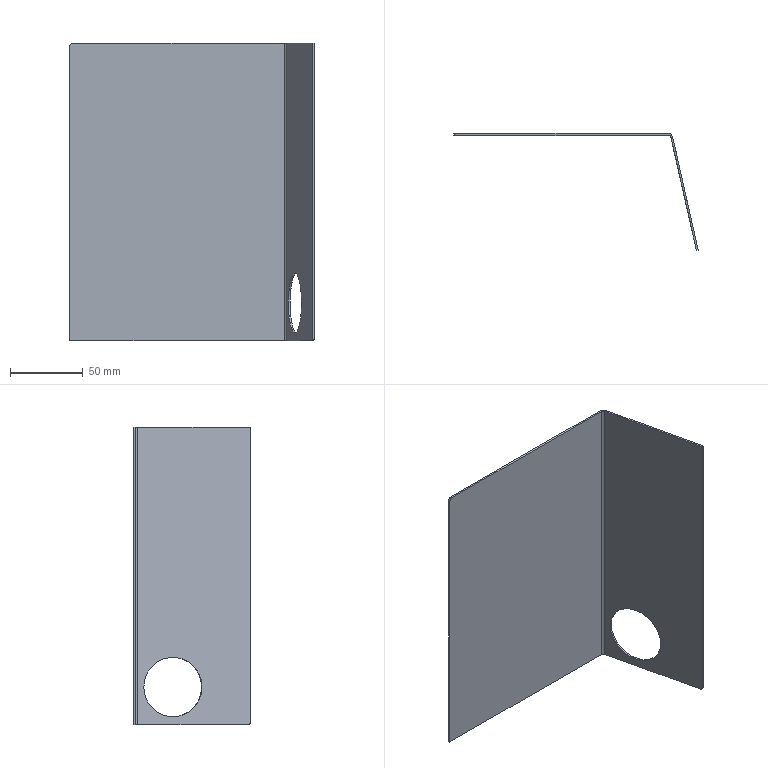Part | SolidWorks | features Fillet 1, FlatPattern 1, ICE 1, SMBaseFlange 1, SheetMetal 1 | 1 solid | 18 faces | box 168 x 80.263 x 204.8 mm | volume 55034 mm3 | plane 12 | cylinder 6 | commonest cylinder face diameters 4 x3 41 x2 6.4 x1
STEP:
#1=CARTESIAN_POINT('',(150.344,-6.995,26.));
#2=VERTEX_POINT('',#1);
#3=CARTESIAN_POINT('',(159.344,-46.995,26.));
#4=VERTEX_POINT('',#3);
#5=CARTESIAN_POINT('',(154.844,-26.995,26.));
#6=DIRECTION('',(-0.9756,-0.2195,0.));
#7=DIRECTION('',(-0.2195,0.9756,0.));
#8=AXIS2_PLACEMENT_3D('',#5,#6,#7);
#9=CIRCLE('',#8,20.5);
#10=EDGE_CURVE('',#2,#4,#9,.T.);
#11=ORIENTED_EDGE('',*,*,#10,.T.);
#12=CARTESIAN_POINT('',(160.515,-46.732,26.));
#13=VERTEX_POINT('',#12);
#14=CARTESIAN_POINT('',(0.5522,-82.723,26.));
#15=DIRECTION('',(0.9756,0.2195,0.));
#16=VECTOR('',#15,1000.);
#17=LINE('',#14,#16);
#18=EDGE_CURVE('',#4,#13,#17,.T.);
#19=ORIENTED_EDGE('',*,*,#18,.T.);
#20=CARTESIAN_POINT('',(151.515,-6.732,26.));
#21=VERTEX_POINT('',#20);
#22=CARTESIAN_POINT('',(156.015,-26.732,26.));
#23=DIRECTION('',(0.9756,0.2195,0.));
#24=DIRECTION('',(-0.2195,0.9756,0.));
#25=AXIS2_PLACEMENT_3D('',#22,#23,#24);
#26=CIRCLE('',#25,20.5);
#27=EDGE_CURVE('',#13,#21,#26,.T.);
#28=ORIENTED_EDGE('',*,*,#27,.T.);
#29=CARTESIAN_POINT('',(-8.448,-42.723,26.));
#30=DIRECTION('',(0.9756,0.2195,0.));
#31=VECTOR('',#30,1000.);
#32=LINE('',#29,#31);
#33=EDGE_CURVE('',#2,#21,#32,.T.);
#34=ORIENTED_EDGE('',*,*,#33,.F.);
#35=EDGE_LOOP('',(#11,#19,#28,#34));
#36=FACE_OUTER_BOUND('',#35,.T.);
#37=CARTESIAN_POINT('',(-3.948,-62.723,26.));
#38=DIRECTION('',(0.9756,0.2195,0.));
#39=DIRECTION('',(-0.2195,0.9756,0.));
#40=AXIS2_PLACEMENT_3D('',#37,#38,#39);
#41=CYLINDRICAL_SURFACE('',#40,20.5);
#42=ADVANCED_FACE('',(#36),#41,.F.);
#43=CARTESIAN_POINT('',(150.562,-2.498,204.8));
#44=VERTEX_POINT('',#43);
#45=CARTESIAN_POINT('',(149.391,-2.761,204.8));
#46=VERTEX_POINT('',#45);
#47=CARTESIAN_POINT('',(150.562,-2.498,204.8));
#48=DIRECTION('',(-0.9756,-0.2195,0.));
#49=VECTOR('',#48,1000.);
#50=LINE('',#47,#49);
#51=EDGE_CURVE('',#44,#46,#50,.T.);
#52=ORIENTED_EDGE('',*,*,#51,.F.);
#53=CARTESIAN_POINT('',(147.44,0.,204.8));
#54=VERTEX_POINT('',#53);
#55=CARTESIAN_POINT('',(147.44,-3.2,204.8));
#56=DIRECTION('',(0.,0.,-1.));
#57=DIRECTION('',(1.,0.,0.));
#58=AXIS2_PLACEMENT_3D('',#55,#56,#57);
#59=CIRCLE('',#58,3.2);
#60=EDGE_CURVE('',#54,#44,#59,.T.);
#61=ORIENTED_EDGE('',*,*,#60,.F.);
#62=CARTESIAN_POINT('',(147.44,-1.2,204.8));
#63=VERTEX_POINT('',#62);
#64=CARTESIAN_POINT('',(147.44,-1.2,204.8));
#65=DIRECTION('',(0.,1.,0.));
#66=VECTOR('',#65,1000.);
#67=LINE('',#64,#66);
#68=EDGE_CURVE('',#63,#54,#67,.T.);
#69=ORIENTED_EDGE('',*,*,#68,.F.);
#70=CARTESIAN_POINT('',(147.44,-3.2,204.8));
#71=DIRECTION('',(0.,0.,-1.));
#72=DIRECTION('',(1.,0.,0.));
#73=AXIS2_PLACEMENT_3D('',#70,#71,#72);
#74=CIRCLE('',#73,2.);
#75=EDGE_CURVE('',#63,#46,#74,.T.);
#76=ORIENTED_EDGE('',*,*,#75,.T.);
#77=EDGE_LOOP('',(#52,#61,#69,#76));
#78=FACE_OUTER_BOUND('',#77,.T.);
#79=CARTESIAN_POINT('',(150.562,-2.498,204.8));
#80=DIRECTION('',(0.,0.,1.));
#81=DIRECTION('',(1.,0.,0.));
#82=AXIS2_PLACEMENT_3D('',#79,#80,#81);
#83=PLANE('',#82);
#84=ADVANCED_FACE('',(#78),#83,.T.);
#85=CARTESIAN_POINT('',(168.,-80.,204.8));
#86=VERTEX_POINT('',#85);
#87=CARTESIAN_POINT('',(150.,0.,204.8));
#88=DIRECTION('',(0.2195,-0.9756,0.));
#89=VECTOR('',#88,1000.);
#90=LINE('',#87,#89);
#91=EDGE_CURVE('',#44,#86,#90,.T.);
#92=ORIENTED_EDGE('',*,*,#91,.F.);
#93=ORIENTED_EDGE('',*,*,#51,.T.);
#94=CARTESIAN_POINT('',(166.829,-80.263,204.8));
#95=VERTEX_POINT('',#94);
#96=CARTESIAN_POINT('',(148.829,-0.2634,204.8));
#97=DIRECTION('',(0.2195,-0.9756,0.));
#98=VECTOR('',#97,1000.);
#99=LINE('',#96,#98);
#100=EDGE_CURVE('',#46,#95,#99,.T.);
#101=ORIENTED_EDGE('',*,*,#100,.T.);
#102=CARTESIAN_POINT('',(168.,-80.,204.8));
#103=DIRECTION('',(-0.9756,-0.2195,0.));
#104=VECTOR('',#103,1000.);
#105=LINE('',#102,#104);
#106=EDGE_CURVE('',#86,#95,#105,.T.);
#107=ORIENTED_EDGE('',*,*,#106,.F.);
#108=EDGE_LOOP('',(#92,#93,#101,#107));
#109=FACE_OUTER_BOUND('',#108,.T.);
#110=CARTESIAN_POINT('',(147.44,-1.2,204.8));
#111=DIRECTION('',(0.,0.,1.));
#112=DIRECTION('',(1.,0.,0.));
#113=AXIS2_PLACEMENT_3D('',#110,#111,#112);
#114=PLANE('',#113);
#115=ADVANCED_FACE('',(#109),#114,.T.);
#116=CARTESIAN_POINT('',(147.44,0.,0.));
#117=VERTEX_POINT('',#116);
#118=CARTESIAN_POINT('',(147.44,-1.2,0.));
#119=VERTEX_POINT('',#118);
#120=CARTESIAN_POINT('',(147.44,0.,0.));
#121=DIRECTION('',(0.,-1.,0.));
#122=VECTOR('',#121,1000.);
#123=LINE('',#120,#122);
#124=EDGE_CURVE('',#117,#119,#123,.T.);
#125=ORIENTED_EDGE('',*,*,#124,.F.);
#126=CARTESIAN_POINT('',(150.562,-2.498,0.));
#127=VERTEX_POINT('',#126);
#128=CARTESIAN_POINT('',(147.44,-3.2,0.));
#129=DIRECTION('',(0.,0.,-1.));
#130=DIRECTION('',(1.,0.,0.));
#131=AXIS2_PLACEMENT_3D('',#128,#129,#130);
#132=CIRCLE('',#131,3.2);
#133=EDGE_CURVE('',#117,#127,#132,.T.);
#134=ORIENTED_EDGE('',*,*,#133,.T.);
#135=CARTESIAN_POINT('',(149.391,-2.761,0.));
#136=VERTEX_POINT('',#135);
#137=CARTESIAN_POINT('',(149.391,-2.761,0.));
#138=DIRECTION('',(0.9756,0.2195,0.));
#139=VECTOR('',#138,1000.);
#140=LINE('',#137,#139);
#141=EDGE_CURVE('',#136,#127,#140,.T.);
#142=ORIENTED_EDGE('',*,*,#141,.F.);
#143=CARTESIAN_POINT('',(147.44,-3.2,0.));
#144=DIRECTION('',(0.,0.,-1.));
#145=DIRECTION('',(1.,0.,0.));
#146=AXIS2_PLACEMENT_3D('',#143,#144,#145);
#147=CIRCLE('',#146,2.);
#148=EDGE_CURVE('',#119,#136,#147,.T.);
#149=ORIENTED_EDGE('',*,*,#148,.F.);
#150=EDGE_LOOP('',(#125,#134,#142,#149));
#151=FACE_OUTER_BOUND('',#150,.T.);
#152=CARTESIAN_POINT('',(147.44,0.,0.));
#153=DIRECTION('',(0.,0.,-1.));
#154=DIRECTION('',(-1.,0.,0.));
#155=AXIS2_PLACEMENT_3D('',#152,#153,#154);
#156=PLANE('',#155);
#157=ADVANCED_FACE('',(#151),#156,.T.);
#158=CARTESIAN_POINT('',(0.,0.,0.));
#159=VERTEX_POINT('',#158);
#160=CARTESIAN_POINT('',(0.,0.,0.));
#161=DIRECTION('',(1.,0.,0.));
#162=VECTOR('',#161,1000.);
#163=LINE('',#160,#162);
#164=EDGE_CURVE('',#159,#117,#163,.T.);
#165=ORIENTED_EDGE('',*,*,#164,.T.);
#166=ORIENTED_EDGE('',*,*,#124,.T.);
#167=CARTESIAN_POINT('',(0.,-1.2,0.));
#168=VERTEX_POINT('',#167);
#169=CARTESIAN_POINT('',(0.,-1.2,0.));
#170=DIRECTION('',(1.,0.,0.));
#171=VECTOR('',#170,1000.);
#172=LINE('',#169,#171);
#173=EDGE_CURVE('',#168,#119,#172,.T.);
#174=ORIENTED_EDGE('',*,*,#173,.F.);
#175=CARTESIAN_POINT('',(0.,-1.2,0.));
#176=DIRECTION('',(0.,1.,0.));
#177=VECTOR('',#176,1000.);
#178=LINE('',#175,#177);
#179=EDGE_CURVE('',#168,#159,#178,.T.);
#180=ORIENTED_EDGE('',*,*,#179,.T.);
#181=EDGE_LOOP('',(#165,#166,#174,#180));
#182=FACE_OUTER_BOUND('',#181,.T.);
#183=CARTESIAN_POINT('',(149.391,-2.761,0.));
#184=DIRECTION('',(0.,0.,-1.));
#185=DIRECTION('',(-1.,0.,0.));
#186=AXIS2_PLACEMENT_3D('',#183,#184,#185);
#187=PLANE('',#186);
#188=ADVANCED_FACE('',(#182),#187,.T.);
#189=ORIENTED_EDGE('',*,*,#10,.F.);
#190=CARTESIAN_POINT('',(154.844,-26.995,26.));
#191=DIRECTION('',(-0.9756,-0.2195,0.));
#192=DIRECTION('',(-0.2195,0.9756,0.));
#193=AXIS2_PLACEMENT_3D('',#190,#191,#192);
#194=CIRCLE('',#193,20.5);
#195=EDGE_CURVE('',#4,#2,#194,.T.);
#196=ORIENTED_EDGE('',*,*,#195,.F.);
#197=EDGE_LOOP('',(#189,#196));
#198=FACE_BOUND('',#197,.T.);
#199=CARTESIAN_POINT('',(166.39,-78.312,0.));
#200=VERTEX_POINT('',#199);
#201=CARTESIAN_POINT('',(148.829,-0.2634,0.));
#202=DIRECTION('',(0.2195,-0.9756,0.));
#203=VECTOR('',#202,1000.);
#204=LINE('',#201,#203);
#205=EDGE_CURVE('',#136,#200,#204,.T.);
#206=ORIENTED_EDGE('',*,*,#205,.T.);
#207=CARTESIAN_POINT('',(166.829,-80.263,2.));
#208=VERTEX_POINT('',#207);
#209=CARTESIAN_POINT('',(166.39,-78.312,2.));
#210=DIRECTION('',(-0.9756,-0.2195,0.));
#211=DIRECTION('',(-0.2195,0.9756,0.));
#212=AXIS2_PLACEMENT_3D('',#209,#210,#211);
#213=CIRCLE('',#212,2.);
#214=EDGE_CURVE('',#200,#208,#213,.T.);
#215=ORIENTED_EDGE('',*,*,#214,.T.);
#216=CARTESIAN_POINT('',(166.829,-80.263,204.8));
#217=DIRECTION('',(0.,0.,-1.));
#218=VECTOR('',#217,1000.);
#219=LINE('',#216,#218);
#220=EDGE_CURVE('',#95,#208,#219,.T.);
#221=ORIENTED_EDGE('',*,*,#220,.F.);
#222=ORIENTED_EDGE('',*,*,#100,.F.);
#223=CARTESIAN_POINT('',(149.391,-2.761,204.8));
#224=DIRECTION('',(0.,0.,-1.));
#225=VECTOR('',#224,1000.);
#226=LINE('',#223,#225);
#227=EDGE_CURVE('',#46,#136,#226,.T.);
#228=ORIENTED_EDGE('',*,*,#227,.T.);
#229=EDGE_LOOP('',(#206,#215,#221,#222,#228));
#230=FACE_OUTER_BOUND('',#229,.T.);
#231=CARTESIAN_POINT('',(148.829,-0.2634,204.8));
#232=DIRECTION('',(0.9756,0.2195,0.));
#233=DIRECTION('',(-0.2195,0.9756,0.));
#234=AXIS2_PLACEMENT_3D('',#231,#232,#233);
#235=PLANE('',#234);
#236=ADVANCED_FACE('',(#198,#230),#235,.F.);
#237=ORIENTED_EDGE('',*,*,#220,.T.);
#238=CARTESIAN_POINT('',(168.,-80.,2.));
#239=VERTEX_POINT('',#238);
#240=CARTESIAN_POINT('',(168.,-80.,2.));
#241=DIRECTION('',(0.9756,0.2195,0.));
#242=VECTOR('',#241,1000.);
#243=LINE('',#240,#242);
#244=EDGE_CURVE('',#208,#239,#243,.T.);
#245=ORIENTED_EDGE('',*,*,#244,.T.);
#246=CARTESIAN_POINT('',(168.,-80.,204.8));
#247=DIRECTION('',(0.,0.,-1.));
#248=VECTOR('',#247,1000.);
#249=LINE('',#246,#248);
#250=EDGE_CURVE('',#86,#239,#249,.T.);
#251=ORIENTED_EDGE('',*,*,#250,.F.);
#252=ORIENTED_EDGE('',*,*,#106,.T.);
#253=EDGE_LOOP('',(#237,#245,#251,#252));
#254=FACE_OUTER_BOUND('',#253,.T.);
#255=CARTESIAN_POINT('',(168.,-80.,204.8));
#256=DIRECTION('',(0.2195,-0.9756,0.));
#257=DIRECTION('',(0.9756,0.2195,0.));
#258=AXIS2_PLACEMENT_3D('',#255,#256,#257);
#259=PLANE('',#258);
#260=ADVANCED_FACE('',(#254),#259,.T.);
#261=CARTESIAN_POINT('',(156.015,-26.732,26.));
#262=DIRECTION('',(0.9756,0.2195,0.));
#263=DIRECTION('',(-0.2195,0.9756,0.));
#264=AXIS2_PLACEMENT_3D('',#261,#262,#263);
#265=CIRCLE('',#264,20.5);
#266=EDGE_CURVE('',#21,#13,#265,.T.);
#267=ORIENTED_EDGE('',*,*,#266,.F.);
#268=ORIENTED_EDGE('',*,*,#27,.F.);
#269=EDGE_LOOP('',(#267,#268));
#270=FACE_BOUND('',#269,.T.);
#271=ORIENTED_EDGE('',*,*,#250,.T.);
#272=CARTESIAN_POINT('',(167.561,-78.049,0.));
#273=VERTEX_POINT('',#272);
#274=CARTESIAN_POINT('',(167.561,-78.049,2.));
#275=DIRECTION('',(0.9756,0.2195,0.));
#276=DIRECTION('',(-0.2195,0.9756,0.));
#277=AXIS2_PLACEMENT_3D('',#274,#275,#276);
#278=CIRCLE('',#277,2.);
#279=EDGE_CURVE('',#239,#273,#278,.T.);
#280=ORIENTED_EDGE('',*,*,#279,.T.);
#281=CARTESIAN_POINT('',(150.,0.,0.));
#282=DIRECTION('',(0.2195,-0.9756,0.));
#283=VECTOR('',#282,1000.);
#284=LINE('',#281,#283);
#285=EDGE_CURVE('',#127,#273,#284,.T.);
#286=ORIENTED_EDGE('',*,*,#285,.F.);
#287=CARTESIAN_POINT('',(150.562,-2.498,204.8));
#288=DIRECTION('',(0.,0.,-1.));
#289=VECTOR('',#288,1000.);
#290=LINE('',#287,#289);
#291=EDGE_CURVE('',#44,#127,#290,.T.);
#292=ORIENTED_EDGE('',*,*,#291,.F.);
#293=ORIENTED_EDGE('',*,*,#91,.T.);
#294=EDGE_LOOP('',(#271,#280,#286,#292,#293));
#295=FACE_OUTER_BOUND('',#294,.T.);
#296=CARTESIAN_POINT('',(150.,0.,204.8));
#297=DIRECTION('',(0.9756,0.2195,0.));
#298=DIRECTION('',(-0.2195,0.9756,0.));
#299=AXIS2_PLACEMENT_3D('',#296,#297,#298);
#300=PLANE('',#299);
#301=ADVANCED_FACE('',(#270,#295),#300,.T.);
#302=ORIENTED_EDGE('',*,*,#133,.F.);
#303=CARTESIAN_POINT('',(147.44,0.,204.8));
#304=DIRECTION('',(0.,0.,-1.));
#305=VECTOR('',#304,1000.);
#306=LINE('',#303,#305);
#307=EDGE_CURVE('',#54,#117,#306,.T.);
#308=ORIENTED_EDGE('',*,*,#307,.F.);
#309=ORIENTED_EDGE('',*,*,#60,.T.);
#310=ORIENTED_EDGE('',*,*,#291,.T.);
#311=EDGE_LOOP('',(#302,#308,#309,#310));
#312=FACE_OUTER_BOUND('',#311,.T.);
#313=CARTESIAN_POINT('',(147.44,-3.2,204.8));
#314=DIRECTION('',(0.,0.,-1.));
#315=DIRECTION('',(-1.,0.,0.));
#316=AXIS2_PLACEMENT_3D('',#313,#314,#315);
#317=CYLINDRICAL_SURFACE('',#316,3.2);
#318=ADVANCED_FACE('',(#312),#317,.T.);
#319=CARTESIAN_POINT('',(0.,0.,202.8));
#320=VERTEX_POINT('',#319);
#321=CARTESIAN_POINT('',(0.,0.,204.8));
#322=DIRECTION('',(0.,0.,-1.));
#323=VECTOR('',#322,1000.);
#324=LINE('',#321,#323);
#325=EDGE_CURVE('',#320,#159,#324,.T.);
#326=ORIENTED_EDGE('',*,*,#325,.F.);
#327=CARTESIAN_POINT('',(2.,0.,204.8));
#328=VERTEX_POINT('',#327);
#329=CARTESIAN_POINT('',(2.,0.,202.8));
#330=DIRECTION('',(0.,1.,0.));
#331=DIRECTION('',(0.,0.,1.));
#332=AXIS2_PLACEMENT_3D('',#329,#330,#331);
#333=CIRCLE('',#332,2.);
#334=EDGE_CURVE('',#320,#328,#333,.T.);
#335=ORIENTED_EDGE('',*,*,#334,.T.);
#336=CARTESIAN_POINT('',(0.,0.,204.8));
#337=DIRECTION('',(1.,0.,0.));
#338=VECTOR('',#337,1000.);
#339=LINE('',#336,#338);
#340=EDGE_CURVE('',#328,#54,#339,.T.);
#341=ORIENTED_EDGE('',*,*,#340,.T.);
#342=ORIENTED_EDGE('',*,*,#307,.T.);
#343=ORIENTED_EDGE('',*,*,#164,.F.);
#344=EDGE_LOOP('',(#326,#335,#341,#342,#343));
#345=FACE_OUTER_BOUND('',#344,.T.);
#346=CARTESIAN_POINT('',(0.,0.,204.8));
#347=DIRECTION('',(0.,1.,0.));
#348=DIRECTION('',(0.,0.,1.));
#349=AXIS2_PLACEMENT_3D('',#346,#347,#348);
#350=PLANE('',#349);
#351=ADVANCED_FACE('',(#345),#350,.T.);
#352=CARTESIAN_POINT('',(0.,-1.2,202.8));
#353=VERTEX_POINT('',#352);
#354=CARTESIAN_POINT('',(0.,-1.2,204.8));
#355=DIRECTION('',(0.,0.,-1.));
#356=VECTOR('',#355,1000.);
#357=LINE('',#354,#356);
#358=EDGE_CURVE('',#353,#168,#357,.T.);
#359=ORIENTED_EDGE('',*,*,#358,.F.);
#360=CARTESIAN_POINT('',(0.,-1.2,202.8));
#361=DIRECTION('',(0.,1.,0.));
#362=VECTOR('',#361,1000.);
#363=LINE('',#360,#362);
#364=EDGE_CURVE('',#353,#320,#363,.T.);
#365=ORIENTED_EDGE('',*,*,#364,.T.);
#366=ORIENTED_EDGE('',*,*,#325,.T.);
#367=ORIENTED_EDGE('',*,*,#179,.F.);
#368=EDGE_LOOP('',(#359,#365,#366,#367));
#369=FACE_OUTER_BOUND('',#368,.T.);
#370=CARTESIAN_POINT('',(0.,-1.2,204.8));
#371=DIRECTION('',(-1.,0.,0.));
#372=DIRECTION('',(0.,0.,1.));
#373=AXIS2_PLACEMENT_3D('',#370,#371,#372);
#374=PLANE('',#373);
#375=ADVANCED_FACE('',(#369),#374,.T.);
#376=CARTESIAN_POINT('',(2.,-1.2,204.8));
#377=VERTEX_POINT('',#376);
#378=CARTESIAN_POINT('',(0.,-1.2,204.8));
#379=DIRECTION('',(1.,0.,0.));
#380=VECTOR('',#379,1000.);
#381=LINE('',#378,#380);
#382=EDGE_CURVE('',#377,#63,#381,.T.);
#383=ORIENTED_EDGE('',*,*,#382,.F.);
#384=CARTESIAN_POINT('',(2.,-1.2,202.8));
#385=DIRECTION('',(0.,-1.,0.));
#386=DIRECTION('',(0.,0.,1.));
#387=AXIS2_PLACEMENT_3D('',#384,#385,#386);
#388=CIRCLE('',#387,2.);
#389=EDGE_CURVE('',#377,#353,#388,.T.);
#390=ORIENTED_EDGE('',*,*,#389,.T.);
#391=ORIENTED_EDGE('',*,*,#358,.T.);
#392=ORIENTED_EDGE('',*,*,#173,.T.);
#393=CARTESIAN_POINT('',(147.44,-1.2,204.8));
#394=DIRECTION('',(0.,0.,-1.));
#395=VECTOR('',#394,1000.);
#396=LINE('',#393,#395);
#397=EDGE_CURVE('',#63,#119,#396,.T.);
#398=ORIENTED_EDGE('',*,*,#397,.F.);
#399=EDGE_LOOP('',(#383,#390,#391,#392,#398));
#400=FACE_OUTER_BOUND('',#399,.T.);
#401=CARTESIAN_POINT('',(0.,-1.2,204.8));
#402=DIRECTION('',(0.,1.,0.));
#403=DIRECTION('',(0.,0.,1.));
#404=AXIS2_PLACEMENT_3D('',#401,#402,#403);
#405=PLANE('',#404);
#406=ADVANCED_FACE('',(#400),#405,.F.);
#407=ORIENTED_EDGE('',*,*,#148,.T.);
#408=ORIENTED_EDGE('',*,*,#227,.F.);
#409=ORIENTED_EDGE('',*,*,#75,.F.);
#410=ORIENTED_EDGE('',*,*,#397,.T.);
#411=EDGE_LOOP('',(#407,#408,#409,#410));
#412=FACE_OUTER_BOUND('',#411,.T.);
#413=CARTESIAN_POINT('',(147.44,-3.2,204.8));
#414=DIRECTION('',(0.,0.,-1.));
#415=DIRECTION('',(-1.,0.,0.));
#416=AXIS2_PLACEMENT_3D('',#413,#414,#415);
#417=CYLINDRICAL_SURFACE('',#416,2.);
#418=ADVANCED_FACE('',(#412),#417,.F.);
#419=ORIENTED_EDGE('',*,*,#340,.F.);
#420=CARTESIAN_POINT('',(2.,-3.2,204.8));
#421=DIRECTION('',(0.,-1.,0.));
#422=VECTOR('',#421,1000.);
#423=LINE('',#420,#422);
#424=EDGE_CURVE('',#328,#377,#423,.T.);
#425=ORIENTED_EDGE('',*,*,#424,.T.);
#426=ORIENTED_EDGE('',*,*,#382,.T.);
#427=ORIENTED_EDGE('',*,*,#68,.T.);
#428=EDGE_LOOP('',(#419,#425,#426,#427));
#429=FACE_OUTER_BOUND('',#428,.T.);
#430=CARTESIAN_POINT('',(147.44,-3.2,204.8));
#431=DIRECTION('',(0.,0.,1.));
#432=DIRECTION('',(1.,0.,0.));
#433=AXIS2_PLACEMENT_3D('',#430,#431,#432);
#434=PLANE('',#433);
#435=ADVANCED_FACE('',(#429),#434,.T.);
#436=ORIENTED_EDGE('',*,*,#285,.T.);
#437=CARTESIAN_POINT('',(166.39,-78.312,0.));
#438=DIRECTION('',(-0.9756,-0.2195,0.));
#439=VECTOR('',#438,1000.);
#440=LINE('',#437,#439);
#441=EDGE_CURVE('',#273,#200,#440,.T.);
#442=ORIENTED_EDGE('',*,*,#441,.T.);
#443=ORIENTED_EDGE('',*,*,#205,.F.);
#444=ORIENTED_EDGE('',*,*,#141,.T.);
#445=EDGE_LOOP('',(#436,#442,#443,#444));
#446=FACE_OUTER_BOUND('',#445,.T.);
#447=CARTESIAN_POINT('',(147.44,-3.2,0.));
#448=DIRECTION('',(0.,0.,1.));
#449=DIRECTION('',(1.,0.,0.));
#450=AXIS2_PLACEMENT_3D('',#447,#448,#449);
#451=PLANE('',#450);
#452=ADVANCED_FACE('',(#446),#451,.F.);
#453=ORIENTED_EDGE('',*,*,#18,.F.);
#454=ORIENTED_EDGE('',*,*,#195,.T.);
#455=ORIENTED_EDGE('',*,*,#33,.T.);
#456=ORIENTED_EDGE('',*,*,#266,.T.);
#457=EDGE_LOOP('',(#453,#454,#455,#456));
#458=FACE_OUTER_BOUND('',#457,.T.);
#459=CARTESIAN_POINT('',(-3.948,-62.723,26.));
#460=DIRECTION('',(0.9756,0.2195,0.));
#461=DIRECTION('',(-0.2195,0.9756,0.));
#462=AXIS2_PLACEMENT_3D('',#459,#460,#461);
#463=CYLINDRICAL_SURFACE('',#462,20.5);
#464=ADVANCED_FACE('',(#458),#463,.F.);
#465=ORIENTED_EDGE('',*,*,#389,.F.);
#466=ORIENTED_EDGE('',*,*,#424,.F.);
#467=ORIENTED_EDGE('',*,*,#334,.F.);
#468=ORIENTED_EDGE('',*,*,#364,.F.);
#469=EDGE_LOOP('',(#465,#466,#467,#468));
#470=FACE_OUTER_BOUND('',#469,.T.);
#471=CARTESIAN_POINT('',(2.,-1.2,202.8));
#472=DIRECTION('',(0.,1.,0.));
#473=DIRECTION('',(0.,0.,1.));
#474=AXIS2_PLACEMENT_3D('',#471,#472,#473);
#475=CYLINDRICAL_SURFACE('',#474,2.);
#476=ADVANCED_FACE('',(#470),#475,.T.);
#477=ORIENTED_EDGE('',*,*,#279,.F.);
#478=ORIENTED_EDGE('',*,*,#244,.F.);
#479=ORIENTED_EDGE('',*,*,#214,.F.);
#480=ORIENTED_EDGE('',*,*,#441,.F.);
#481=EDGE_LOOP('',(#477,#478,#479,#480));
#482=FACE_OUTER_BOUND('',#481,.T.);
#483=CARTESIAN_POINT('',(164.439,-78.751,2.));
#484=DIRECTION('',(0.9756,0.2195,0.));
#485=DIRECTION('',(-0.2195,0.9756,0.));
#486=AXIS2_PLACEMENT_3D('',#483,#484,#485);
#487=CYLINDRICAL_SURFACE('',#486,2.);
#488=ADVANCED_FACE('',(#482),#487,.T.);
#489=CLOSED_SHELL('',(#42,#84,#115,#157,#188,#236,#260,#301,#318,#351,#375,#406,#418,#435,#452,#464,#476,#488));
#490=MANIFOLD_SOLID_BREP('',#489);
#491=CARTESIAN_POINT('',(0.,0.,0.));
#492=DIRECTION('',(0.,0.,1.));
#493=DIRECTION('',(1.,0.,0.));
#494=AXIS2_PLACEMENT_3D('',#491,#492,#493);
#495=(LENGTH_UNIT()NAMED_UNIT(*)SI_UNIT(.MILLI.,.METRE.));
#496=UNCERTAINTY_MEASURE_WITH_UNIT(LENGTH_MEASURE(0.00001),#495,'','');
#497=(NAMED_UNIT(*)PLANE_ANGLE_UNIT()SI_UNIT($,.RADIAN.));
#498=(NAMED_UNIT(*)SI_UNIT($,.STERADIAN.)SOLID_ANGLE_UNIT());
#499=(GEOMETRIC_REPRESENTATION_CONTEXT(3)GLOBAL_UNCERTAINTY_ASSIGNED_CONTEXT((#496))GLOBAL_UNIT_ASSIGNED_CONTEXT((#495,#497,#498))REPRESENTATION_CONTEXT('',''));
#500=ADVANCED_BREP_SHAPE_REPRESENTATION('',(#490,#494),#499);